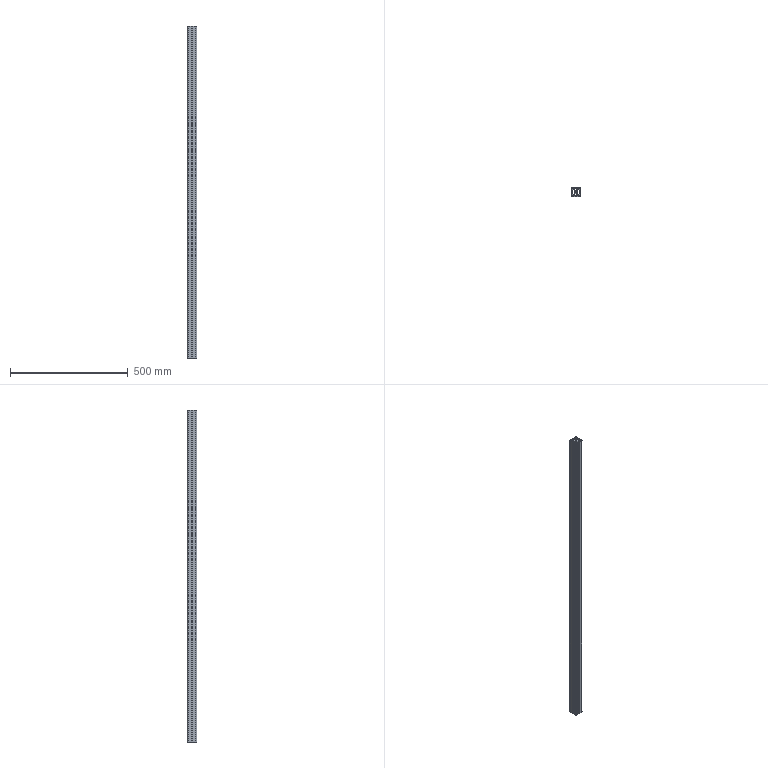Part | STEP file | 40x40-1410 | 1 solid | 88 faces | box 40 x 40 x 1410 mm | volume 992565 mm3 | plane 78 | cylinder 10 | commonest cylinder face diameters 4 x4 10 x4 6.8 x2